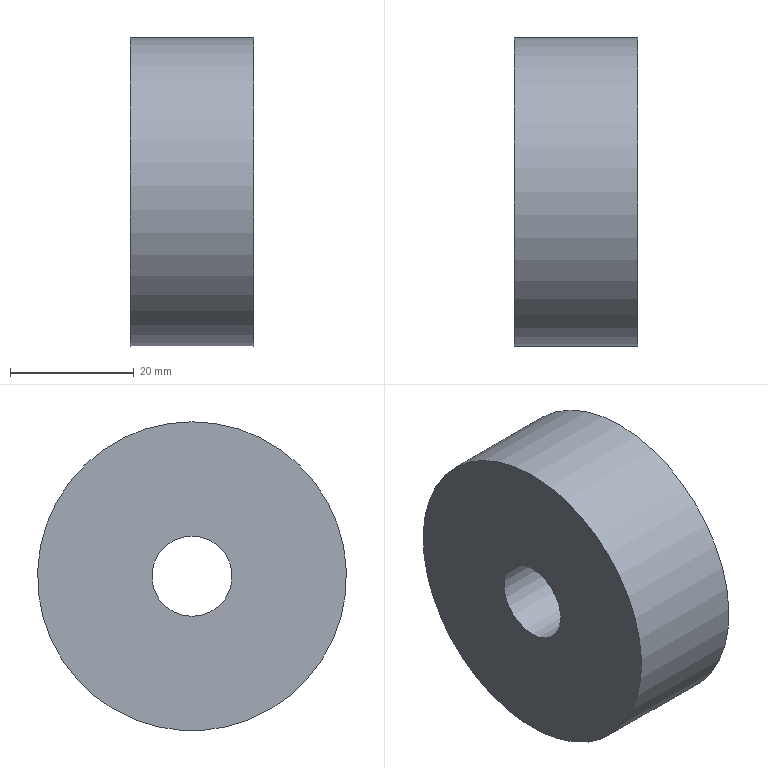Part | NX | features solid 2 | 1 solid | 6 faces | box 20 x 50 x 50 mm | volume 34801 mm3 | cylinder 3 | plane 3 | commonest cylinder face diameters 13 x1 20 x1 50 x1
STEP:
#1=CARTESIAN_POINT('',(555.,930.,-150.));
#2=VERTEX_POINT('',#1);
#3=CARTESIAN_POINT('',(555.,930.,-175.));
#4=DIRECTION('',(-1.,0.,0.));
#5=DIRECTION('',(0.,0.,1.));
#6=AXIS2_PLACEMENT_3D('',#3,#4,#5);
#7=CIRCLE('',#6,25.);
#8=EDGE_CURVE('',#2,#2,#7,.T.);
#9=ORIENTED_EDGE('',*,*,#8,.F.);
#10=EDGE_LOOP('',(#9));
#11=FACE_BOUND('',#10,.T.);
#12=CARTESIAN_POINT('',(575.,930.,-150.));
#13=VERTEX_POINT('',#12);
#14=CARTESIAN_POINT('',(575.,930.,-175.));
#15=DIRECTION('',(-1.,0.,0.));
#16=DIRECTION('',(0.,0.,1.));
#17=AXIS2_PLACEMENT_3D('',#14,#15,#16);
#18=CIRCLE('',#17,25.);
#19=EDGE_CURVE('',#13,#13,#18,.T.);
#20=ORIENTED_EDGE('',*,*,#19,.T.);
#21=EDGE_LOOP('',(#20));
#22=FACE_BOUND('',#21,.T.);
#23=CARTESIAN_POINT('',(555.,930.,-175.));
#24=DIRECTION('',(1.,0.,0.));
#25=DIRECTION('',(0.,0.,1.));
#26=AXIS2_PLACEMENT_3D('',#23,#24,#25);
#27=CYLINDRICAL_SURFACE('',#26,25.);
#28=ADVANCED_FACE('',(#11,#22),#27,.T.);
#29=CARTESIAN_POINT('',(555.,930.,-181.5));
#30=VERTEX_POINT('',#29);
#31=CARTESIAN_POINT('',(555.,930.,-175.));
#32=DIRECTION('',(-1.,0.,0.));
#33=DIRECTION('',(0.,0.,-1.));
#34=AXIS2_PLACEMENT_3D('',#31,#32,#33);
#35=CIRCLE('',#34,6.5);
#36=EDGE_CURVE('',#30,#30,#35,.T.);
#37=ORIENTED_EDGE('',*,*,#36,.F.);
#38=EDGE_LOOP('',(#37));
#39=FACE_BOUND('',#38,.T.);
#40=ORIENTED_EDGE('',*,*,#8,.T.);
#41=EDGE_LOOP('',(#40));
#42=FACE_BOUND('',#41,.T.);
#43=CARTESIAN_POINT('',(555.,930.,-175.));
#44=DIRECTION('',(-1.,0.,0.));
#45=DIRECTION('',(0.,0.,-1.));
#46=AXIS2_PLACEMENT_3D('',#43,#44,#45);
#47=PLANE('',#46);
#48=ADVANCED_FACE('',(#39,#42),#47,.T.);
#49=CARTESIAN_POINT('',(575.,930.,-185.));
#50=VERTEX_POINT('',#49);
#51=CARTESIAN_POINT('',(575.,930.,-175.));
#52=DIRECTION('',(-1.,0.,0.));
#53=DIRECTION('',(0.,0.,-1.));
#54=AXIS2_PLACEMENT_3D('',#51,#52,#53);
#55=CIRCLE('',#54,10.);
#56=EDGE_CURVE('',#50,#50,#55,.T.);
#57=ORIENTED_EDGE('',*,*,#56,.T.);
#58=EDGE_LOOP('',(#57));
#59=FACE_BOUND('',#58,.T.);
#60=ORIENTED_EDGE('',*,*,#19,.F.);
#61=EDGE_LOOP('',(#60));
#62=FACE_BOUND('',#61,.T.);
#63=CARTESIAN_POINT('',(575.,930.,-175.));
#64=DIRECTION('',(-1.,0.,0.));
#65=DIRECTION('',(0.,0.,-1.));
#66=AXIS2_PLACEMENT_3D('',#63,#64,#65);
#67=PLANE('',#66);
#68=ADVANCED_FACE('',(#59,#62),#67,.F.);
#69=CARTESIAN_POINT('',(565.,930.,-181.5));
#70=VERTEX_POINT('',#69);
#71=CARTESIAN_POINT('',(565.,930.,-175.));
#72=DIRECTION('',(-1.,0.,0.));
#73=DIRECTION('',(0.,0.,-1.));
#74=AXIS2_PLACEMENT_3D('',#71,#72,#73);
#75=CIRCLE('',#74,6.5);
#76=EDGE_CURVE('',#70,#70,#75,.T.);
#77=ORIENTED_EDGE('',*,*,#76,.T.);
#78=EDGE_LOOP('',(#77));
#79=FACE_BOUND('',#78,.T.);
#80=CARTESIAN_POINT('',(565.,930.,-185.));
#81=VERTEX_POINT('',#80);
#82=CARTESIAN_POINT('',(565.,930.,-175.));
#83=DIRECTION('',(-1.,0.,0.));
#84=DIRECTION('',(0.,0.,-1.));
#85=AXIS2_PLACEMENT_3D('',#82,#83,#84);
#86=CIRCLE('',#85,10.);
#87=EDGE_CURVE('',#81,#81,#86,.T.);
#88=ORIENTED_EDGE('',*,*,#87,.F.);
#89=EDGE_LOOP('',(#88));
#90=FACE_BOUND('',#89,.T.);
#91=CARTESIAN_POINT('',(565.,930.,-175.));
#92=DIRECTION('',(-1.,0.,0.));
#93=DIRECTION('',(0.,0.,-1.));
#94=AXIS2_PLACEMENT_3D('',#91,#92,#93);
#95=PLANE('',#94);
#96=ADVANCED_FACE('',(#79,#90),#95,.F.);
#97=ORIENTED_EDGE('',*,*,#87,.T.);
#98=EDGE_LOOP('',(#97));
#99=FACE_BOUND('',#98,.T.);
#100=ORIENTED_EDGE('',*,*,#56,.F.);
#101=EDGE_LOOP('',(#100));
#102=FACE_BOUND('',#101,.T.);
#103=CARTESIAN_POINT('',(575.,930.,-175.));
#104=DIRECTION('',(-1.,0.,0.));
#105=DIRECTION('',(0.,0.,-1.));
#106=AXIS2_PLACEMENT_3D('',#103,#104,#105);
#107=CYLINDRICAL_SURFACE('',#106,10.);
#108=ADVANCED_FACE('',(#99,#102),#107,.F.);
#109=ORIENTED_EDGE('',*,*,#36,.T.);
#110=EDGE_LOOP('',(#109));
#111=FACE_BOUND('',#110,.T.);
#112=ORIENTED_EDGE('',*,*,#76,.F.);
#113=EDGE_LOOP('',(#112));
#114=FACE_BOUND('',#113,.T.);
#115=CARTESIAN_POINT('',(565.,930.,-175.));
#116=DIRECTION('',(-1.,0.,0.));
#117=DIRECTION('',(0.,0.,-1.));
#118=AXIS2_PLACEMENT_3D('',#115,#116,#117);
#119=CYLINDRICAL_SURFACE('',#118,6.5);
#120=ADVANCED_FACE('',(#111,#114),#119,.F.);
#121=CLOSED_SHELL('',(#28,#48,#68,#96,#108,#120));
#122=MANIFOLD_SOLID_BREP('',#121);
#123=(LENGTH_UNIT()NAMED_UNIT(*)SI_UNIT(.MILLI.,.METRE.));
#124=UNCERTAINTY_MEASURE_WITH_UNIT(LENGTH_MEASURE(0.00001),#123,'','');
#125=(NAMED_UNIT(*)PLANE_ANGLE_UNIT()SI_UNIT($,.RADIAN.));
#126=(NAMED_UNIT(*)SI_UNIT($,.STERADIAN.)SOLID_ANGLE_UNIT());
#127=(GEOMETRIC_REPRESENTATION_CONTEXT(3)GLOBAL_UNCERTAINTY_ASSIGNED_CONTEXT((#124))GLOBAL_UNIT_ASSIGNED_CONTEXT((#123,#125,#126))REPRESENTATION_CONTEXT('',''));
#128=ADVANCED_BREP_SHAPE_REPRESENTATION('',(#122),#127);